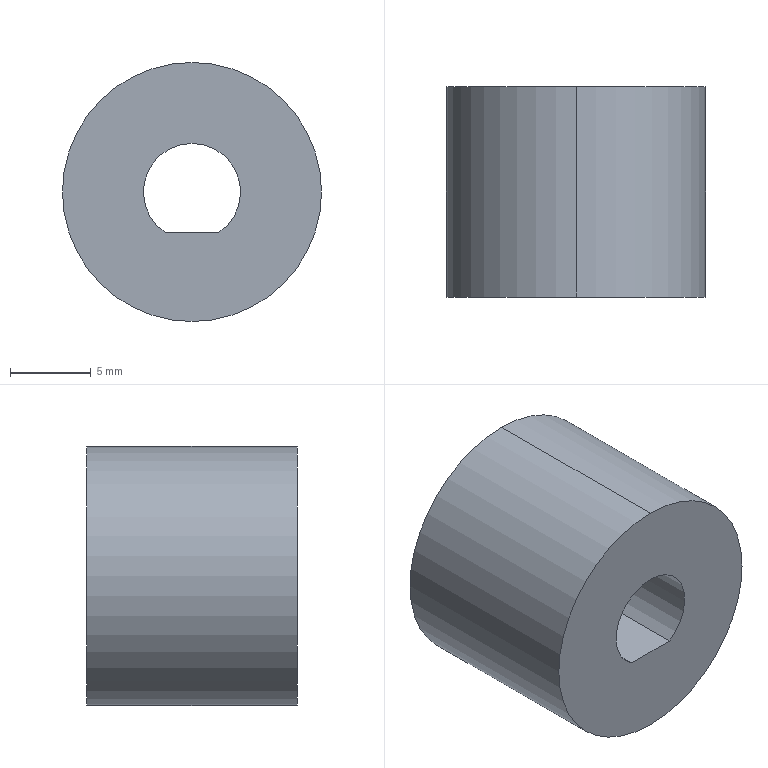Part | 1 solid | 7 faces | box 16 x 13 x 16 mm | volume 2261 mm3 | cylinder 4 | plane 3 | commonest cylinder face diameters 6 x2 16 x2
STEP:
#1=CARTESIAN_POINT('',(0.,0.,3.));
#2=VERTEX_POINT('',#1);
#3=CARTESIAN_POINT('',(1.658,0.,-2.5));
#4=VERTEX_POINT('',#3);
#5=CARTESIAN_POINT('',(0.,0.,0.));
#6=DIRECTION('',(0.,1.,0.));
#7=DIRECTION('',(0.,0.,1.));
#8=AXIS2_PLACEMENT_3D('',#5,#6,#7);
#9=CIRCLE('',#8,3.);
#10=EDGE_CURVE('',#2,#4,#9,.T.);
#11=ORIENTED_EDGE('',*,*,#10,.F.);
#12=CARTESIAN_POINT('',(0.,13.,3.));
#13=VERTEX_POINT('',#12);
#14=CARTESIAN_POINT('',(0.,0.,3.));
#15=DIRECTION('',(0.,1.,0.));
#16=VECTOR('',#15,1000.);
#17=LINE('',#14,#16);
#18=EDGE_CURVE('',#2,#13,#17,.T.);
#19=ORIENTED_EDGE('',*,*,#18,.T.);
#20=CARTESIAN_POINT('',(1.658,13.,-2.5));
#21=VERTEX_POINT('',#20);
#22=CARTESIAN_POINT('',(0.,13.,0.));
#23=DIRECTION('',(0.,1.,0.));
#24=DIRECTION('',(0.,0.,1.));
#25=AXIS2_PLACEMENT_3D('',#22,#23,#24);
#26=CIRCLE('',#25,3.);
#27=EDGE_CURVE('',#13,#21,#26,.T.);
#28=ORIENTED_EDGE('',*,*,#27,.T.);
#29=CARTESIAN_POINT('',(1.658,0.,-2.5));
#30=DIRECTION('',(0.,1.,0.));
#31=VECTOR('',#30,1000.);
#32=LINE('',#29,#31);
#33=EDGE_CURVE('',#4,#21,#32,.T.);
#34=ORIENTED_EDGE('',*,*,#33,.F.);
#35=EDGE_LOOP('',(#11,#19,#28,#34));
#36=FACE_OUTER_BOUND('',#35,.T.);
#37=CARTESIAN_POINT('',(0.,0.,0.));
#38=DIRECTION('',(0.,1.,0.));
#39=DIRECTION('',(0.,0.,1.));
#40=AXIS2_PLACEMENT_3D('',#37,#38,#39);
#41=CYLINDRICAL_SURFACE('',#40,3.);
#42=ADVANCED_FACE('',(#36),#41,.F.);
#43=CARTESIAN_POINT('',(0.,13.,8.));
#44=VERTEX_POINT('',#43);
#45=CARTESIAN_POINT('',(0.,13.,-8.));
#46=VERTEX_POINT('',#45);
#47=CARTESIAN_POINT('',(0.,13.,0.));
#48=DIRECTION('',(0.,1.,0.));
#49=DIRECTION('',(0.,0.,1.));
#50=AXIS2_PLACEMENT_3D('',#47,#48,#49);
#51=CIRCLE('',#50,8.);
#52=EDGE_CURVE('',#44,#46,#51,.T.);
#53=ORIENTED_EDGE('',*,*,#52,.F.);
#54=CARTESIAN_POINT('',(0.,0.,8.));
#55=VERTEX_POINT('',#54);
#56=CARTESIAN_POINT('',(0.,13.,8.));
#57=DIRECTION('',(0.,-1.,0.));
#58=VECTOR('',#57,1000.);
#59=LINE('',#56,#58);
#60=EDGE_CURVE('',#44,#55,#59,.T.);
#61=ORIENTED_EDGE('',*,*,#60,.T.);
#62=CARTESIAN_POINT('',(0.,0.,-8.));
#63=VERTEX_POINT('',#62);
#64=CARTESIAN_POINT('',(0.,0.,0.));
#65=DIRECTION('',(0.,1.,0.));
#66=DIRECTION('',(0.,0.,1.));
#67=AXIS2_PLACEMENT_3D('',#64,#65,#66);
#68=CIRCLE('',#67,8.);
#69=EDGE_CURVE('',#55,#63,#68,.T.);
#70=ORIENTED_EDGE('',*,*,#69,.T.);
#71=CARTESIAN_POINT('',(0.,13.,-8.));
#72=DIRECTION('',(0.,-1.,0.));
#73=VECTOR('',#72,1000.);
#74=LINE('',#71,#73);
#75=EDGE_CURVE('',#46,#63,#74,.T.);
#76=ORIENTED_EDGE('',*,*,#75,.F.);
#77=EDGE_LOOP('',(#53,#61,#70,#76));
#78=FACE_OUTER_BOUND('',#77,.T.);
#79=CARTESIAN_POINT('',(0.,13.,0.));
#80=DIRECTION('',(0.,-1.,0.));
#81=DIRECTION('',(0.,0.,-1.));
#82=AXIS2_PLACEMENT_3D('',#79,#80,#81);
#83=CYLINDRICAL_SURFACE('',#82,8.);
#84=ADVANCED_FACE('',(#78),#83,.T.);
#85=ORIENTED_EDGE('',*,*,#60,.F.);
#86=CARTESIAN_POINT('',(0.,13.,0.));
#87=DIRECTION('',(0.,1.,0.));
#88=DIRECTION('',(0.,0.,1.));
#89=AXIS2_PLACEMENT_3D('',#86,#87,#88);
#90=CIRCLE('',#89,8.);
#91=EDGE_CURVE('',#46,#44,#90,.T.);
#92=ORIENTED_EDGE('',*,*,#91,.F.);
#93=ORIENTED_EDGE('',*,*,#75,.T.);
#94=CARTESIAN_POINT('',(0.,0.,0.));
#95=DIRECTION('',(0.,1.,0.));
#96=DIRECTION('',(0.,0.,1.));
#97=AXIS2_PLACEMENT_3D('',#94,#95,#96);
#98=CIRCLE('',#97,8.);
#99=EDGE_CURVE('',#63,#55,#98,.T.);
#100=ORIENTED_EDGE('',*,*,#99,.T.);
#101=EDGE_LOOP('',(#85,#92,#93,#100));
#102=FACE_OUTER_BOUND('',#101,.T.);
#103=CARTESIAN_POINT('',(0.,13.,0.));
#104=DIRECTION('',(0.,-1.,0.));
#105=DIRECTION('',(0.,0.,-1.));
#106=AXIS2_PLACEMENT_3D('',#103,#104,#105);
#107=CYLINDRICAL_SURFACE('',#106,8.);
#108=ADVANCED_FACE('',(#102),#107,.T.);
#109=CARTESIAN_POINT('',(-1.658,13.,-2.5));
#110=VERTEX_POINT('',#109);
#111=CARTESIAN_POINT('',(0.,13.,0.));
#112=DIRECTION('',(0.,1.,0.));
#113=DIRECTION('',(0.,0.,1.));
#114=AXIS2_PLACEMENT_3D('',#111,#112,#113);
#115=CIRCLE('',#114,3.);
#116=EDGE_CURVE('',#110,#13,#115,.T.);
#117=ORIENTED_EDGE('',*,*,#116,.F.);
#118=CARTESIAN_POINT('',(-1.658,13.,-2.5));
#119=DIRECTION('',(-1.,0.,0.));
#120=VECTOR('',#119,1000.);
#121=LINE('',#118,#120);
#122=EDGE_CURVE('',#21,#110,#121,.T.);
#123=ORIENTED_EDGE('',*,*,#122,.F.);
#124=ORIENTED_EDGE('',*,*,#27,.F.);
#125=EDGE_LOOP('',(#117,#123,#124));
#126=FACE_BOUND('',#125,.T.);
#127=ORIENTED_EDGE('',*,*,#91,.T.);
#128=ORIENTED_EDGE('',*,*,#52,.T.);
#129=EDGE_LOOP('',(#127,#128));
#130=FACE_OUTER_BOUND('',#129,.T.);
#131=CARTESIAN_POINT('',(0.,13.,0.));
#132=DIRECTION('',(0.,1.,0.));
#133=DIRECTION('',(0.,0.,1.));
#134=AXIS2_PLACEMENT_3D('',#131,#132,#133);
#135=PLANE('',#134);
#136=ADVANCED_FACE('',(#126,#130),#135,.T.);
#137=CARTESIAN_POINT('',(-1.658,0.,-2.5));
#138=VERTEX_POINT('',#137);
#139=CARTESIAN_POINT('',(-1.658,0.,-2.5));
#140=DIRECTION('',(-1.,0.,0.));
#141=VECTOR('',#140,1000.);
#142=LINE('',#139,#141);
#143=EDGE_CURVE('',#4,#138,#142,.T.);
#144=ORIENTED_EDGE('',*,*,#143,.T.);
#145=CARTESIAN_POINT('',(0.,0.,0.));
#146=DIRECTION('',(0.,1.,0.));
#147=DIRECTION('',(0.,0.,1.));
#148=AXIS2_PLACEMENT_3D('',#145,#146,#147);
#149=CIRCLE('',#148,3.);
#150=EDGE_CURVE('',#138,#2,#149,.T.);
#151=ORIENTED_EDGE('',*,*,#150,.T.);
#152=ORIENTED_EDGE('',*,*,#10,.T.);
#153=EDGE_LOOP('',(#144,#151,#152));
#154=FACE_BOUND('',#153,.T.);
#155=ORIENTED_EDGE('',*,*,#99,.F.);
#156=ORIENTED_EDGE('',*,*,#69,.F.);
#157=EDGE_LOOP('',(#155,#156));
#158=FACE_OUTER_BOUND('',#157,.T.);
#159=CARTESIAN_POINT('',(0.,0.,0.));
#160=DIRECTION('',(0.,1.,0.));
#161=DIRECTION('',(0.,0.,1.));
#162=AXIS2_PLACEMENT_3D('',#159,#160,#161);
#163=PLANE('',#162);
#164=ADVANCED_FACE('',(#154,#158),#163,.F.);
#165=ORIENTED_EDGE('',*,*,#18,.F.);
#166=ORIENTED_EDGE('',*,*,#150,.F.);
#167=CARTESIAN_POINT('',(-1.658,0.,-2.5));
#168=DIRECTION('',(0.,1.,0.));
#169=VECTOR('',#168,1000.);
#170=LINE('',#167,#169);
#171=EDGE_CURVE('',#138,#110,#170,.T.);
#172=ORIENTED_EDGE('',*,*,#171,.T.);
#173=ORIENTED_EDGE('',*,*,#116,.T.);
#174=EDGE_LOOP('',(#165,#166,#172,#173));
#175=FACE_OUTER_BOUND('',#174,.T.);
#176=CARTESIAN_POINT('',(0.,0.,0.));
#177=DIRECTION('',(0.,1.,0.));
#178=DIRECTION('',(0.,0.,1.));
#179=AXIS2_PLACEMENT_3D('',#176,#177,#178);
#180=CYLINDRICAL_SURFACE('',#179,3.);
#181=ADVANCED_FACE('',(#175),#180,.F.);
#182=ORIENTED_EDGE('',*,*,#122,.T.);
#183=ORIENTED_EDGE('',*,*,#171,.F.);
#184=ORIENTED_EDGE('',*,*,#143,.F.);
#185=ORIENTED_EDGE('',*,*,#33,.T.);
#186=EDGE_LOOP('',(#182,#183,#184,#185));
#187=FACE_OUTER_BOUND('',#186,.T.);
#188=CARTESIAN_POINT('',(-1.658,0.,-2.5));
#189=DIRECTION('',(0.,0.,-1.));
#190=DIRECTION('',(-1.,0.,0.));
#191=AXIS2_PLACEMENT_3D('',#188,#189,#190);
#192=PLANE('',#191);
#193=ADVANCED_FACE('',(#187),#192,.F.);
#194=CLOSED_SHELL('',(#42,#84,#108,#136,#164,#181,#193));
#195=MANIFOLD_SOLID_BREP('',#194);
#196=CARTESIAN_POINT('',(0.,0.,0.));
#197=DIRECTION('',(0.,0.,1.));
#198=DIRECTION('',(1.,0.,0.));
#199=AXIS2_PLACEMENT_3D('',#196,#197,#198);
#200=(LENGTH_UNIT()NAMED_UNIT(*)SI_UNIT(.MILLI.,.METRE.));
#201=UNCERTAINTY_MEASURE_WITH_UNIT(LENGTH_MEASURE(0.00001),#200,'','');
#202=(NAMED_UNIT(*)PLANE_ANGLE_UNIT()SI_UNIT($,.RADIAN.));
#203=(NAMED_UNIT(*)SI_UNIT($,.STERADIAN.)SOLID_ANGLE_UNIT());
#204=(GEOMETRIC_REPRESENTATION_CONTEXT(3)GLOBAL_UNCERTAINTY_ASSIGNED_CONTEXT((#201))GLOBAL_UNIT_ASSIGNED_CONTEXT((#200,#202,#203))REPRESENTATION_CONTEXT('',''));
#205=ADVANCED_BREP_SHAPE_REPRESENTATION('',(#195,#199),#204);